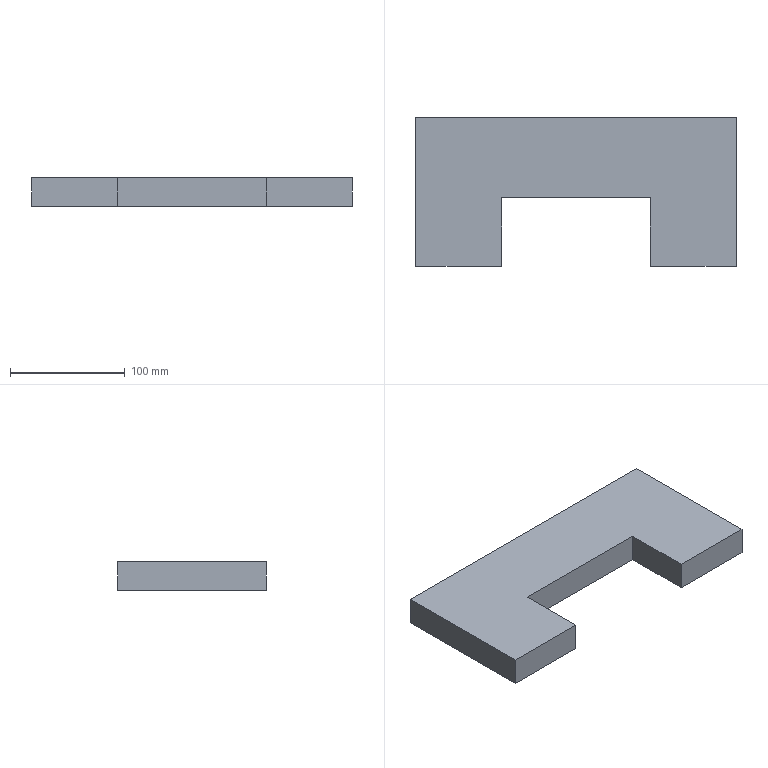Part | SolidWorks | features Extrusion 1 | 1 solid | 10 faces | box 280 x 130 x 25 mm | volume 715000 mm3 | plane 10
STEP:
#1=CARTESIAN_POINT('',(65.,-65.,0.));
#2=VERTEX_POINT('',#1);
#3=CARTESIAN_POINT('',(140.,-65.,0.));
#4=VERTEX_POINT('',#3);
#5=CARTESIAN_POINT('',(65.,-65.,0.));
#6=DIRECTION('',(1.,0.,0.));
#7=VECTOR('',#6,1000.);
#8=LINE('',#5,#7);
#9=EDGE_CURVE('',#2,#4,#8,.T.);
#10=ORIENTED_EDGE('',*,*,#9,.T.);
#11=CARTESIAN_POINT('',(140.,-65.,25.));
#12=VERTEX_POINT('',#11);
#13=CARTESIAN_POINT('',(140.,-65.,25.));
#14=DIRECTION('',(0.,0.,-1.));
#15=VECTOR('',#14,1000.);
#16=LINE('',#13,#15);
#17=EDGE_CURVE('',#12,#4,#16,.T.);
#18=ORIENTED_EDGE('',*,*,#17,.F.);
#19=CARTESIAN_POINT('',(65.,-65.,25.));
#20=VERTEX_POINT('',#19);
#21=CARTESIAN_POINT('',(65.,-65.,25.));
#22=DIRECTION('',(1.,0.,0.));
#23=VECTOR('',#22,1000.);
#24=LINE('',#21,#23);
#25=EDGE_CURVE('',#20,#12,#24,.T.);
#26=ORIENTED_EDGE('',*,*,#25,.F.);
#27=CARTESIAN_POINT('',(65.,-65.,25.));
#28=DIRECTION('',(0.,0.,-1.));
#29=VECTOR('',#28,1000.);
#30=LINE('',#27,#29);
#31=EDGE_CURVE('',#20,#2,#30,.T.);
#32=ORIENTED_EDGE('',*,*,#31,.T.);
#33=EDGE_LOOP('',(#10,#18,#26,#32));
#34=FACE_OUTER_BOUND('',#33,.T.);
#35=CARTESIAN_POINT('',(65.,-65.,25.));
#36=DIRECTION('',(0.,1.,0.));
#37=DIRECTION('',(0.,0.,1.));
#38=AXIS2_PLACEMENT_3D('',#35,#36,#37);
#39=PLANE('',#38);
#40=ADVANCED_FACE('',(#34),#39,.F.);
#41=CARTESIAN_POINT('',(140.,65.,0.));
#42=VERTEX_POINT('',#41);
#43=CARTESIAN_POINT('',(140.,65.,0.));
#44=DIRECTION('',(0.,1.,0.));
#45=VECTOR('',#44,1000.);
#46=LINE('',#43,#45);
#47=EDGE_CURVE('',#4,#42,#46,.T.);
#48=ORIENTED_EDGE('',*,*,#47,.T.);
#49=CARTESIAN_POINT('',(140.,65.,25.));
#50=VERTEX_POINT('',#49);
#51=CARTESIAN_POINT('',(140.,65.,25.));
#52=DIRECTION('',(0.,0.,-1.));
#53=VECTOR('',#52,1000.);
#54=LINE('',#51,#53);
#55=EDGE_CURVE('',#50,#42,#54,.T.);
#56=ORIENTED_EDGE('',*,*,#55,.F.);
#57=CARTESIAN_POINT('',(140.,65.,25.));
#58=DIRECTION('',(0.,1.,0.));
#59=VECTOR('',#58,1000.);
#60=LINE('',#57,#59);
#61=EDGE_CURVE('',#12,#50,#60,.T.);
#62=ORIENTED_EDGE('',*,*,#61,.F.);
#63=ORIENTED_EDGE('',*,*,#17,.T.);
#64=EDGE_LOOP('',(#48,#56,#62,#63));
#65=FACE_OUTER_BOUND('',#64,.T.);
#66=CARTESIAN_POINT('',(140.,65.,25.));
#67=DIRECTION('',(-1.,0.,0.));
#68=DIRECTION('',(0.,-1.,0.));
#69=AXIS2_PLACEMENT_3D('',#66,#67,#68);
#70=PLANE('',#69);
#71=ADVANCED_FACE('',(#65),#70,.F.);
#72=CARTESIAN_POINT('',(-140.,65.,0.));
#73=VERTEX_POINT('',#72);
#74=CARTESIAN_POINT('',(-140.,65.,0.));
#75=DIRECTION('',(-1.,0.,0.));
#76=VECTOR('',#75,1000.);
#77=LINE('',#74,#76);
#78=EDGE_CURVE('',#42,#73,#77,.T.);
#79=ORIENTED_EDGE('',*,*,#78,.T.);
#80=CARTESIAN_POINT('',(-140.,65.,25.));
#81=VERTEX_POINT('',#80);
#82=CARTESIAN_POINT('',(-140.,65.,25.));
#83=DIRECTION('',(0.,0.,-1.));
#84=VECTOR('',#83,1000.);
#85=LINE('',#82,#84);
#86=EDGE_CURVE('',#81,#73,#85,.T.);
#87=ORIENTED_EDGE('',*,*,#86,.F.);
#88=CARTESIAN_POINT('',(-140.,65.,25.));
#89=DIRECTION('',(-1.,0.,0.));
#90=VECTOR('',#89,1000.);
#91=LINE('',#88,#90);
#92=EDGE_CURVE('',#50,#81,#91,.T.);
#93=ORIENTED_EDGE('',*,*,#92,.F.);
#94=ORIENTED_EDGE('',*,*,#55,.T.);
#95=EDGE_LOOP('',(#79,#87,#93,#94));
#96=FACE_OUTER_BOUND('',#95,.T.);
#97=CARTESIAN_POINT('',(-140.,65.,25.));
#98=DIRECTION('',(0.,-1.,0.));
#99=DIRECTION('',(0.,0.,-1.));
#100=AXIS2_PLACEMENT_3D('',#97,#98,#99);
#101=PLANE('',#100);
#102=ADVANCED_FACE('',(#96),#101,.F.);
#103=CARTESIAN_POINT('',(-140.,-65.,0.));
#104=VERTEX_POINT('',#103);
#105=CARTESIAN_POINT('',(-140.,65.,0.));
#106=DIRECTION('',(0.,-1.,0.));
#107=VECTOR('',#106,1000.);
#108=LINE('',#105,#107);
#109=EDGE_CURVE('',#73,#104,#108,.T.);
#110=ORIENTED_EDGE('',*,*,#109,.T.);
#111=CARTESIAN_POINT('',(-140.,-65.,25.));
#112=VERTEX_POINT('',#111);
#113=CARTESIAN_POINT('',(-140.,-65.,25.));
#114=DIRECTION('',(0.,0.,-1.));
#115=VECTOR('',#114,1000.);
#116=LINE('',#113,#115);
#117=EDGE_CURVE('',#112,#104,#116,.T.);
#118=ORIENTED_EDGE('',*,*,#117,.F.);
#119=CARTESIAN_POINT('',(-140.,65.,25.));
#120=DIRECTION('',(0.,-1.,0.));
#121=VECTOR('',#120,1000.);
#122=LINE('',#119,#121);
#123=EDGE_CURVE('',#81,#112,#122,.T.);
#124=ORIENTED_EDGE('',*,*,#123,.F.);
#125=ORIENTED_EDGE('',*,*,#86,.T.);
#126=EDGE_LOOP('',(#110,#118,#124,#125));
#127=FACE_OUTER_BOUND('',#126,.T.);
#128=CARTESIAN_POINT('',(-140.,65.,25.));
#129=DIRECTION('',(1.,0.,0.));
#130=DIRECTION('',(0.,1.,0.));
#131=AXIS2_PLACEMENT_3D('',#128,#129,#130);
#132=PLANE('',#131);
#133=ADVANCED_FACE('',(#127),#132,.F.);
#134=CARTESIAN_POINT('',(-65.,-65.,0.));
#135=VERTEX_POINT('',#134);
#136=CARTESIAN_POINT('',(-140.,-65.,0.));
#137=DIRECTION('',(1.,0.,0.));
#138=VECTOR('',#137,1000.);
#139=LINE('',#136,#138);
#140=EDGE_CURVE('',#104,#135,#139,.T.);
#141=ORIENTED_EDGE('',*,*,#140,.T.);
#142=CARTESIAN_POINT('',(-65.,-65.,25.));
#143=VERTEX_POINT('',#142);
#144=CARTESIAN_POINT('',(-65.,-65.,25.));
#145=DIRECTION('',(0.,0.,-1.));
#146=VECTOR('',#145,1000.);
#147=LINE('',#144,#146);
#148=EDGE_CURVE('',#143,#135,#147,.T.);
#149=ORIENTED_EDGE('',*,*,#148,.F.);
#150=CARTESIAN_POINT('',(-140.,-65.,25.));
#151=DIRECTION('',(1.,0.,0.));
#152=VECTOR('',#151,1000.);
#153=LINE('',#150,#152);
#154=EDGE_CURVE('',#112,#143,#153,.T.);
#155=ORIENTED_EDGE('',*,*,#154,.F.);
#156=ORIENTED_EDGE('',*,*,#117,.T.);
#157=EDGE_LOOP('',(#141,#149,#155,#156));
#158=FACE_OUTER_BOUND('',#157,.T.);
#159=CARTESIAN_POINT('',(-140.,-65.,25.));
#160=DIRECTION('',(0.,1.,0.));
#161=DIRECTION('',(0.,0.,1.));
#162=AXIS2_PLACEMENT_3D('',#159,#160,#161);
#163=PLANE('',#162);
#164=ADVANCED_FACE('',(#158),#163,.F.);
#165=CARTESIAN_POINT('',(-65.,-5.,0.));
#166=VERTEX_POINT('',#165);
#167=CARTESIAN_POINT('',(-65.,-5.,0.));
#168=DIRECTION('',(0.,1.,0.));
#169=VECTOR('',#168,1000.);
#170=LINE('',#167,#169);
#171=EDGE_CURVE('',#135,#166,#170,.T.);
#172=ORIENTED_EDGE('',*,*,#171,.T.);
#173=CARTESIAN_POINT('',(-65.,-5.,25.));
#174=VERTEX_POINT('',#173);
#175=CARTESIAN_POINT('',(-65.,-5.,25.));
#176=DIRECTION('',(0.,0.,-1.));
#177=VECTOR('',#176,1000.);
#178=LINE('',#175,#177);
#179=EDGE_CURVE('',#174,#166,#178,.T.);
#180=ORIENTED_EDGE('',*,*,#179,.F.);
#181=CARTESIAN_POINT('',(-65.,-5.,25.));
#182=DIRECTION('',(0.,1.,0.));
#183=VECTOR('',#182,1000.);
#184=LINE('',#181,#183);
#185=EDGE_CURVE('',#143,#174,#184,.T.);
#186=ORIENTED_EDGE('',*,*,#185,.F.);
#187=ORIENTED_EDGE('',*,*,#148,.T.);
#188=EDGE_LOOP('',(#172,#180,#186,#187));
#189=FACE_OUTER_BOUND('',#188,.T.);
#190=CARTESIAN_POINT('',(-65.,-5.,25.));
#191=DIRECTION('',(-1.,0.,0.));
#192=DIRECTION('',(0.,0.,1.));
#193=AXIS2_PLACEMENT_3D('',#190,#191,#192);
#194=PLANE('',#193);
#195=ADVANCED_FACE('',(#189),#194,.F.);
#196=CARTESIAN_POINT('',(65.,-5.,0.));
#197=VERTEX_POINT('',#196);
#198=CARTESIAN_POINT('',(-65.,-5.,0.));
#199=DIRECTION('',(1.,0.,0.));
#200=VECTOR('',#199,1000.);
#201=LINE('',#198,#200);
#202=EDGE_CURVE('',#166,#197,#201,.T.);
#203=ORIENTED_EDGE('',*,*,#202,.T.);
#204=CARTESIAN_POINT('',(65.,-5.,25.));
#205=VERTEX_POINT('',#204);
#206=CARTESIAN_POINT('',(65.,-5.,25.));
#207=DIRECTION('',(0.,0.,-1.));
#208=VECTOR('',#207,1000.);
#209=LINE('',#206,#208);
#210=EDGE_CURVE('',#205,#197,#209,.T.);
#211=ORIENTED_EDGE('',*,*,#210,.F.);
#212=CARTESIAN_POINT('',(-65.,-5.,25.));
#213=DIRECTION('',(1.,0.,0.));
#214=VECTOR('',#213,1000.);
#215=LINE('',#212,#214);
#216=EDGE_CURVE('',#174,#205,#215,.T.);
#217=ORIENTED_EDGE('',*,*,#216,.F.);
#218=ORIENTED_EDGE('',*,*,#179,.T.);
#219=EDGE_LOOP('',(#203,#211,#217,#218));
#220=FACE_OUTER_BOUND('',#219,.T.);
#221=CARTESIAN_POINT('',(-65.,-5.,25.));
#222=DIRECTION('',(0.,1.,0.));
#223=DIRECTION('',(0.,0.,1.));
#224=AXIS2_PLACEMENT_3D('',#221,#222,#223);
#225=PLANE('',#224);
#226=ADVANCED_FACE('',(#220),#225,.F.);
#227=CARTESIAN_POINT('',(65.,-5.,0.));
#228=DIRECTION('',(0.,-1.,0.));
#229=VECTOR('',#228,1000.);
#230=LINE('',#227,#229);
#231=EDGE_CURVE('',#197,#2,#230,.T.);
#232=ORIENTED_EDGE('',*,*,#231,.T.);
#233=ORIENTED_EDGE('',*,*,#31,.F.);
#234=CARTESIAN_POINT('',(65.,-5.,25.));
#235=DIRECTION('',(0.,-1.,0.));
#236=VECTOR('',#235,1000.);
#237=LINE('',#234,#236);
#238=EDGE_CURVE('',#205,#20,#237,.T.);
#239=ORIENTED_EDGE('',*,*,#238,.F.);
#240=ORIENTED_EDGE('',*,*,#210,.T.);
#241=EDGE_LOOP('',(#232,#233,#239,#240));
#242=FACE_OUTER_BOUND('',#241,.T.);
#243=CARTESIAN_POINT('',(65.,-5.,25.));
#244=DIRECTION('',(1.,0.,0.));
#245=DIRECTION('',(0.,0.,-1.));
#246=AXIS2_PLACEMENT_3D('',#243,#244,#245);
#247=PLANE('',#246);
#248=ADVANCED_FACE('',(#242),#247,.F.);
#249=ORIENTED_EDGE('',*,*,#25,.T.);
#250=ORIENTED_EDGE('',*,*,#61,.T.);
#251=ORIENTED_EDGE('',*,*,#92,.T.);
#252=ORIENTED_EDGE('',*,*,#123,.T.);
#253=ORIENTED_EDGE('',*,*,#154,.T.);
#254=ORIENTED_EDGE('',*,*,#185,.T.);
#255=ORIENTED_EDGE('',*,*,#216,.T.);
#256=ORIENTED_EDGE('',*,*,#238,.T.);
#257=EDGE_LOOP('',(#249,#250,#251,#252,#253,#254,#255,#256));
#258=FACE_OUTER_BOUND('',#257,.T.);
#259=CARTESIAN_POINT('',(0.,0.,25.));
#260=DIRECTION('',(0.,0.,-1.));
#261=DIRECTION('',(-1.,0.,0.));
#262=AXIS2_PLACEMENT_3D('',#259,#260,#261);
#263=PLANE('',#262);
#264=ADVANCED_FACE('',(#258),#263,.F.);
#265=ORIENTED_EDGE('',*,*,#9,.F.);
#266=ORIENTED_EDGE('',*,*,#231,.F.);
#267=ORIENTED_EDGE('',*,*,#202,.F.);
#268=ORIENTED_EDGE('',*,*,#171,.F.);
#269=ORIENTED_EDGE('',*,*,#140,.F.);
#270=ORIENTED_EDGE('',*,*,#109,.F.);
#271=ORIENTED_EDGE('',*,*,#78,.F.);
#272=ORIENTED_EDGE('',*,*,#47,.F.);
#273=EDGE_LOOP('',(#265,#266,#267,#268,#269,#270,#271,#272));
#274=FACE_OUTER_BOUND('',#273,.T.);
#275=CARTESIAN_POINT('',(0.,0.,0.));
#276=DIRECTION('',(0.,0.,-1.));
#277=DIRECTION('',(-1.,0.,0.));
#278=AXIS2_PLACEMENT_3D('',#275,#276,#277);
#279=PLANE('',#278);
#280=ADVANCED_FACE('',(#274),#279,.T.);
#281=CLOSED_SHELL('',(#40,#71,#102,#133,#164,#195,#226,#248,#264,#280));
#282=MANIFOLD_SOLID_BREP('',#281);
#283=CARTESIAN_POINT('',(0.,0.,0.));
#284=DIRECTION('',(0.,0.,1.));
#285=DIRECTION('',(1.,0.,0.));
#286=AXIS2_PLACEMENT_3D('',#283,#284,#285);
#287=(LENGTH_UNIT()NAMED_UNIT(*)SI_UNIT(.MILLI.,.METRE.));
#288=UNCERTAINTY_MEASURE_WITH_UNIT(LENGTH_MEASURE(0.00001),#287,'','');
#289=(NAMED_UNIT(*)PLANE_ANGLE_UNIT()SI_UNIT($,.RADIAN.));
#290=(NAMED_UNIT(*)SI_UNIT($,.STERADIAN.)SOLID_ANGLE_UNIT());
#291=(GEOMETRIC_REPRESENTATION_CONTEXT(3)GLOBAL_UNCERTAINTY_ASSIGNED_CONTEXT((#288))GLOBAL_UNIT_ASSIGNED_CONTEXT((#287,#289,#290))REPRESENTATION_CONTEXT('',''));
#292=ADVANCED_BREP_SHAPE_REPRESENTATION('',(#282,#286),#291);